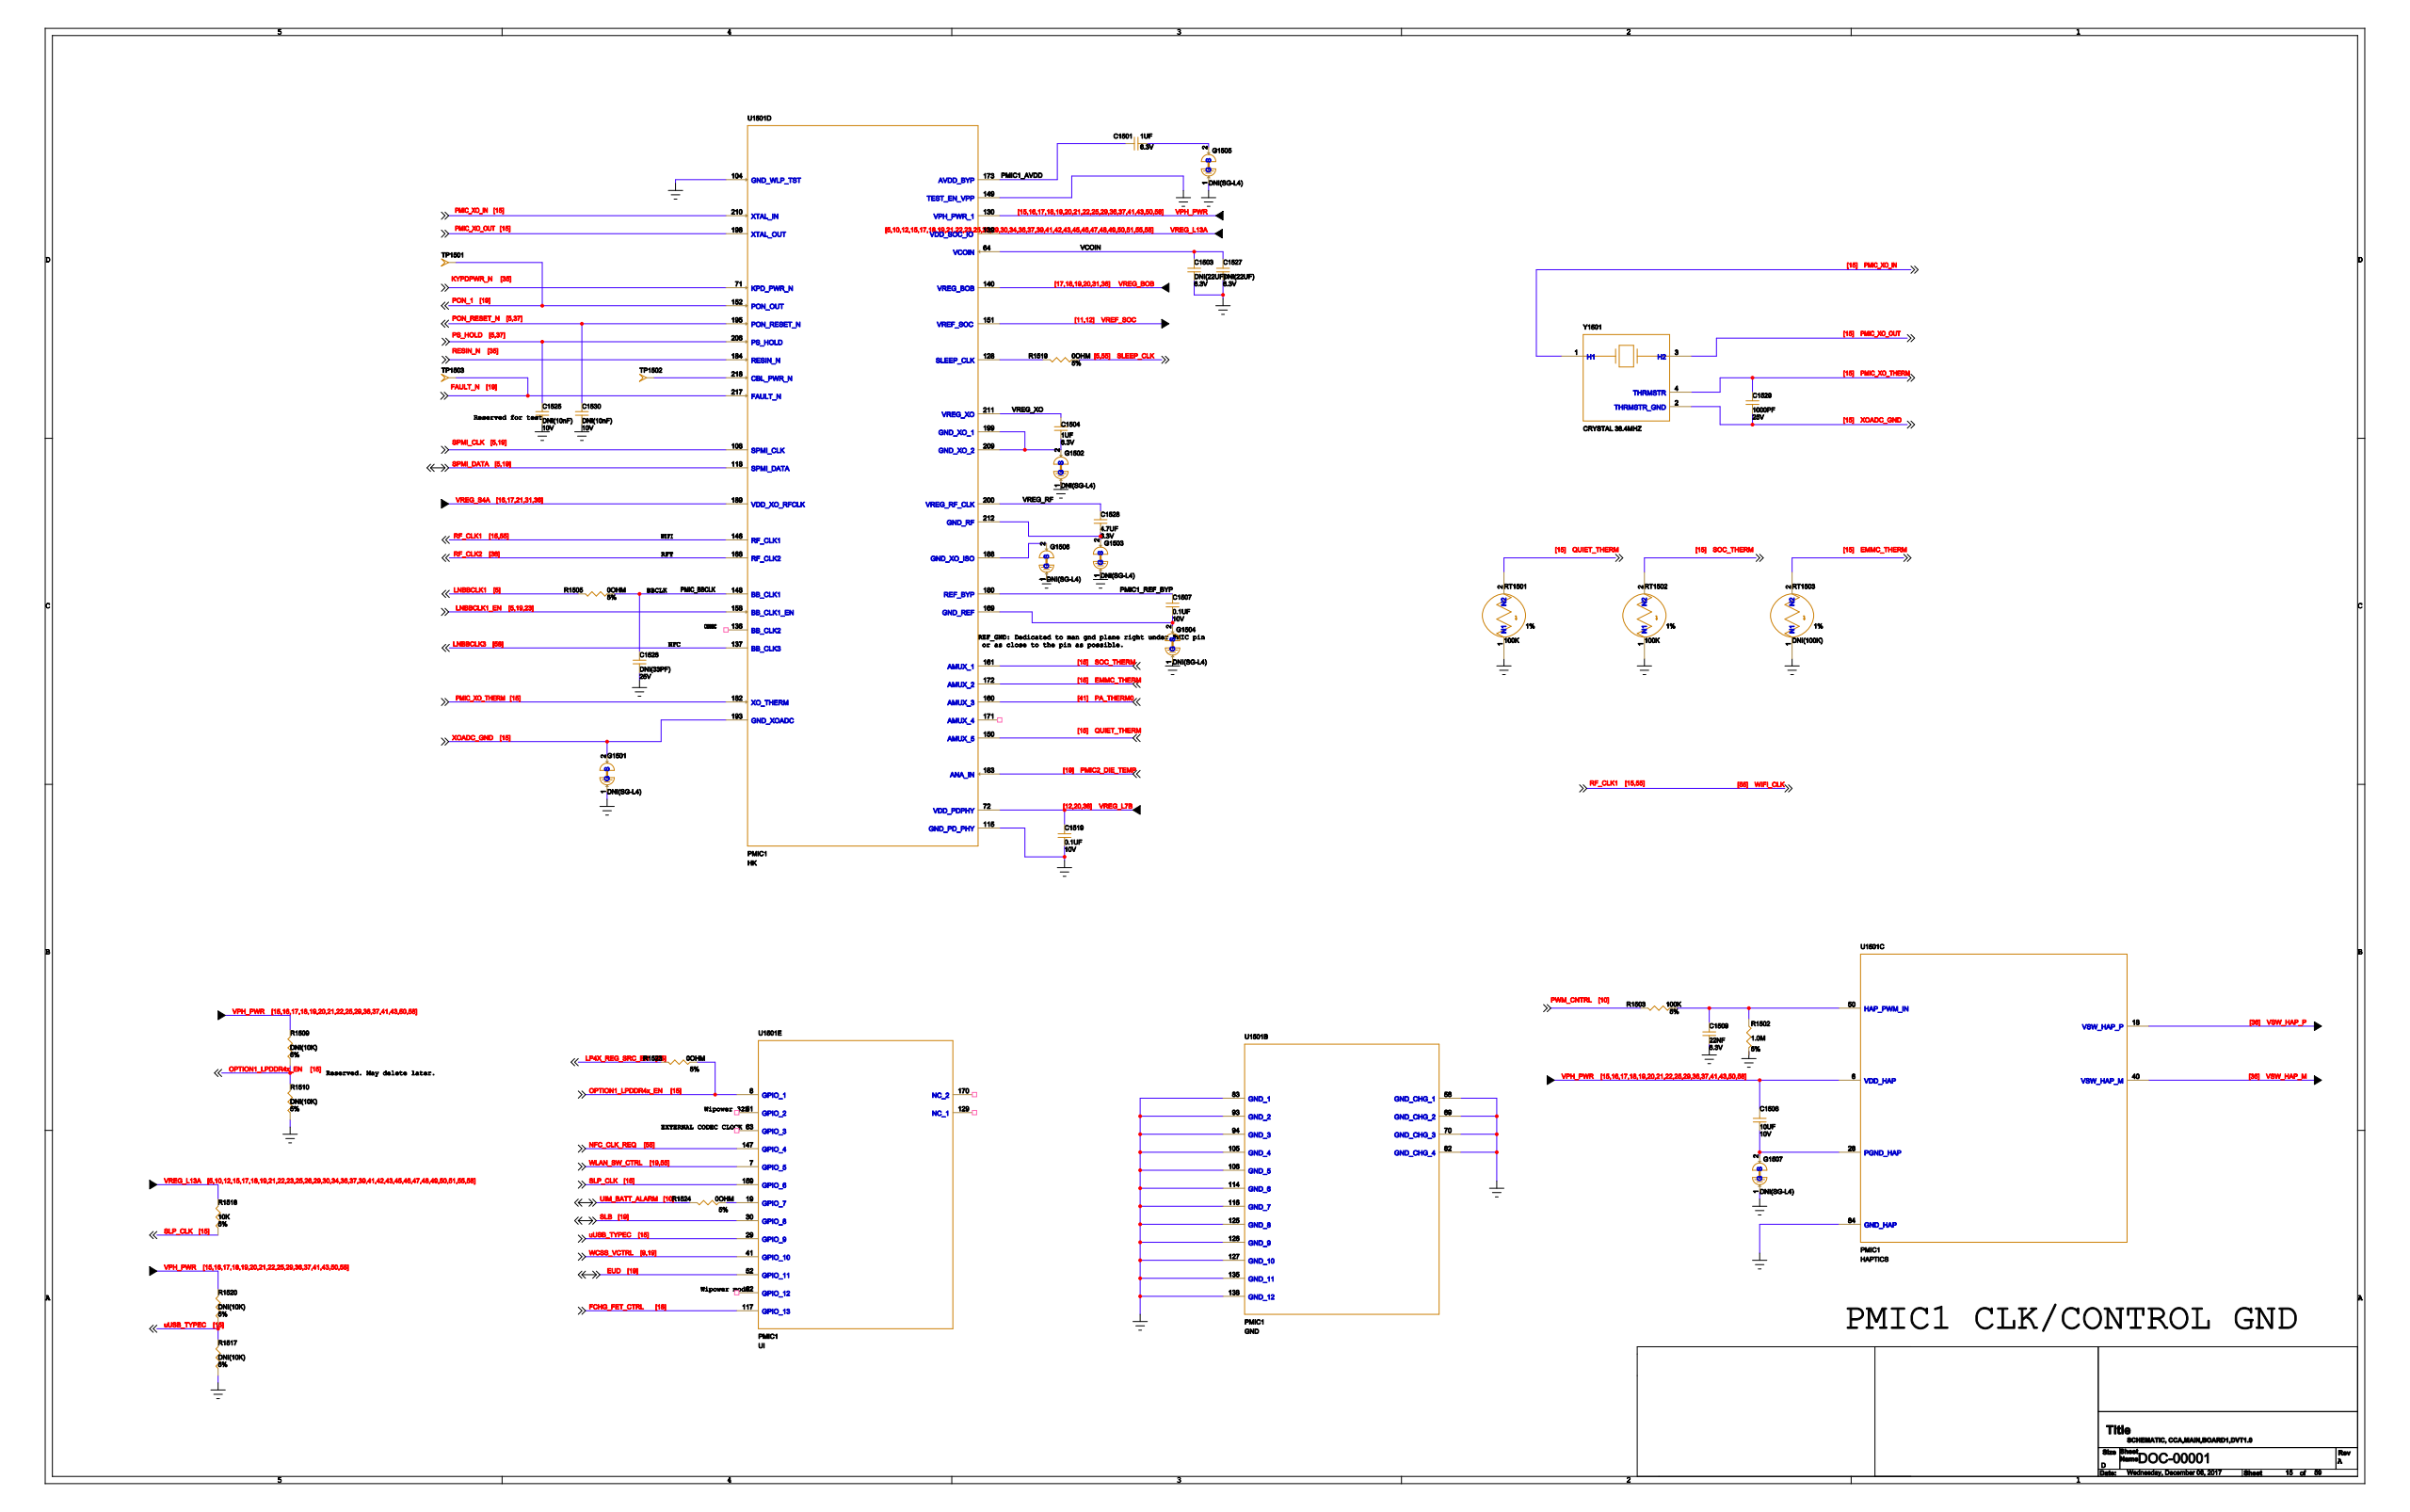Circuit board | KiCad | 1657 parts | 1365 nets | one sheet of the schematic
Parts on this sheet (reference | value | footprint):
C1501
C1503
C1504
C1507
C1508
C1509
C1519
C1525
C1526
C1527
C1528
C1529
C1530
G1501
G1502
G1503
G1504
G1505
G1506
G1507
R1502
R1503
R1505
R1509
R1510
R1517
R1518
R1519
R1520
R1523
R1524
RT1501
RT1502
RT1503
TP1501
TP1502
TP1503
U1501
Y1501
Nets of these parts (net: part-pin ...):
GND: C1503-1 C1509-1 C1519-1 C1525-2 C1526-2 C1527-1 C1530-2 G1501-1 G1502-1 G1503-1 G1504-1 G1505-1 G1506-1 G1507-1 R1502-1 R1510-2 R1517-2 RT1501-1 RT1502-1 RT1503-1 U1501-58 U1501-69 U1501-70 U1501-82 U1501-83 U1501-84 U1501-93 U1501-94 U1501-104 U1501-105 U1501-106 U1501-114 U1501-115 U1501-116 U1501-125 U1501-126 U1501-127 U1501-135 U1501-138 U1501-149
VREG_L13A: R1518-1 U1501-139
N20085253: C1504-1 G1502-2 U1501-199 U1501-209
VPH_PWR: C1508-2 R1509-1 R1520-1 U1501-3 U1501-6 U1501-15 U1501-20 U1501-25 U1501-37 U1501-42 U1501-47 U1501-55 U1501-130
LNBBCLK1_EN: U1501-158
VSW_HAP_M: U1501-40
VREG_BOB: U1501-140
SOC_THERM: RT1502-2 U1501-161
VREG_L7B: C1519-2 U1501-72
SPMI_CLK: U1501-108
PON_RESET_N: C1530-1 U1501-195
UIM_BATT_ALARM: R1524-1
WLAN_SW_CTRL: U1501-7
SLEEP_CLK: R1519-2
N20085367: G1506-2 U1501-188
P4X_REG_SRC_EN: R1523-1
FCHG_FET_CTRL: U1501-117
N20087505: C1508-1 G1507-2 U1501-28
PS_HOLD: C1525-1 U1501-206
VREG_S4A: U1501-189
N20085314: C1507-1 G1504-2 U1501-169
PWM_CNTRL: R1503-1
EMMC_THERM: RT1503-2 U1501-172
VSW_HAP_P: U1501-18
N20085288: C1528-2 G1503-2 U1501-212
RF_CLK1: U1501-146
VREF_SOC: U1501-151
LNBBCLK1: R1505-2
SPMI_DATA: U1501-118
WCSS_VCTRL: U1501-41
XOADC_GND: C1529-2 G1501-2 Y1501-2 U1501-193
N20085428: R1519-1 U1501-128
N20085194: C1501-2 G1505-2
SLP_CLK: R1518-2 U1501-159
LNBBCLK3: U1501-137
UUSB_TYPEC: R1517-1 R1520-2 U1501-29
VREG_XO: C1504-2 U1501-211
PMIC_BBCLK: C1526-1 R1505-1 U1501-148
PMIC_XO_THERM: C1529-1 Y1501-4 U1501-182
ON1_LPDDR4X_EN: R1509-2 R1510-1 R1523-2 U1501-8
PA_THERM0: U1501-160
EUD: U1501-52
N20085304: TP1502-1 U1501-218
NFC_CLK_REQ: U1501-147
KYPDPWR_N: U1501-71
QUIET_THERM: RT1501-2 U1501-150
FAULT_N: TP1503-1 U1501-217
N20087487: C1509-2 R1502-2 R1503-2 U1501-50
VREG_RF: C1528-1 U1501-200
PMIC1_AVDD: C1501-1 U1501-173
PON_1: TP1501-1 U1501-152
PMIC2_DIE_TEMP: U1501-183
SLB: U1501-30
RESIN_N: U1501-184
VCOIN: C1503-2 C1527-2 U1501-64
N23467574: R1524-2 U1501-19
RF_CLK2: U1501-168
PMIC1_REF_BYP: C1507-2 U1501-180
PMIC_XO_OUT: Y1501-3 U1501-198
PMIC_XO_IN: Y1501-1 U1501-210